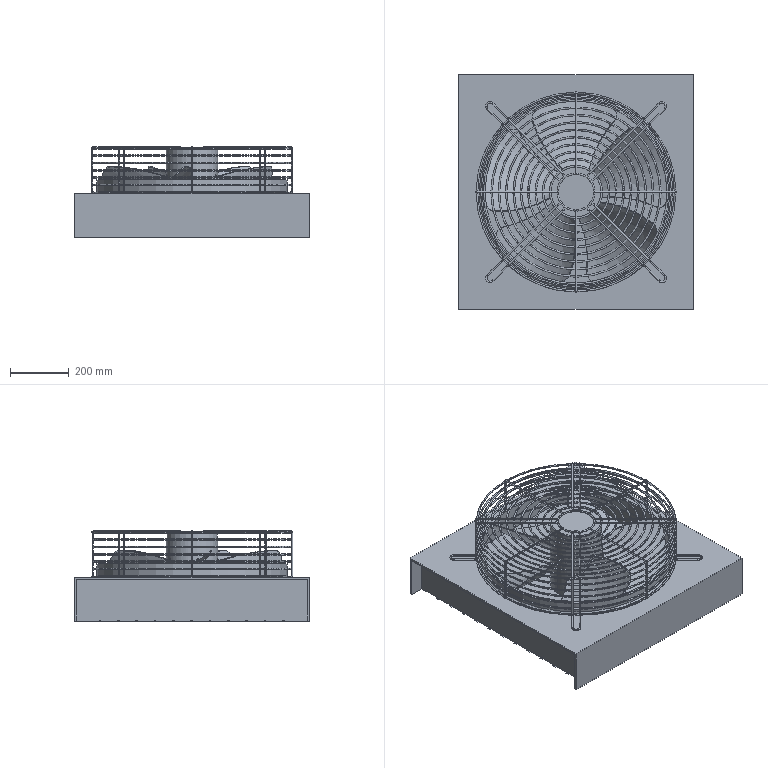Part | SolidWorks | features BaseBody 44, ICE 1 | 5 solids | 587 faces | box 800 x 800 x 307.5 mm | volume 29684405 mm3 | spline 302 | cylinder 219 | plane 60 | torus 6 | commonest cylinder face diameters 5 x160 27.5 x33 50 x6 75 x6 620 x6 175 x4